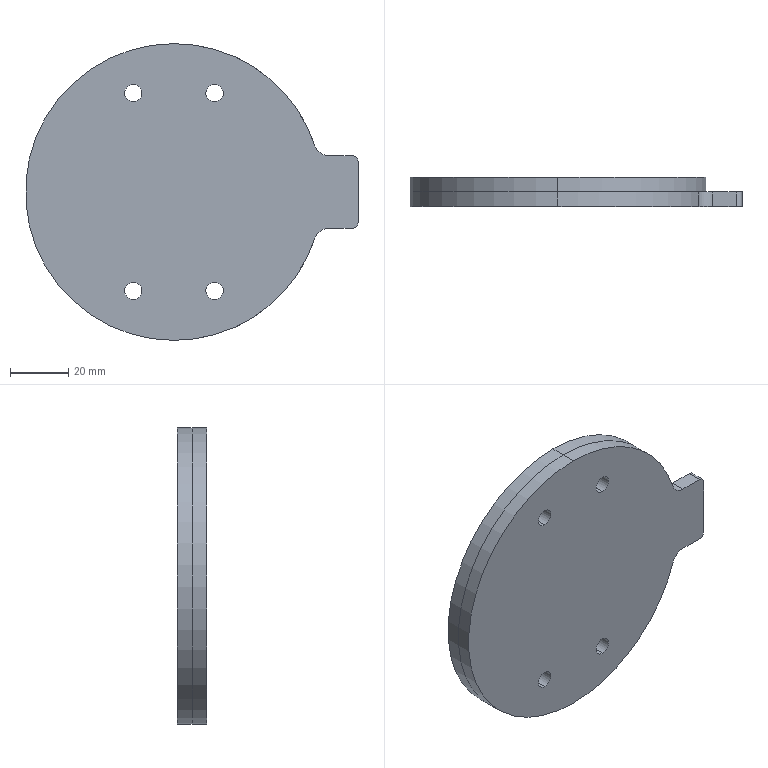Part | SolidWorks | features ICE 4, Extrusion 1, Fillet 1 | 2 solids | 41 faces | box 114.307 x 10 x 102 mm | volume 82051 mm3 | cylinder 31 | plane 10 | commonest cylinder face diameters 6 x16 8 x6 102 x5 4 x2 10 x2
STEP:
#1=CARTESIAN_POINT('',(-14.,0.,-37.));
#2=VERTEX_POINT('',#1);
#3=CARTESIAN_POINT('',(-14.,0.,-31.));
#4=VERTEX_POINT('',#3);
#5=CARTESIAN_POINT('',(-14.,0.,-34.));
#6=DIRECTION('',(0.,1.,0.));
#7=DIRECTION('',(0.,0.,1.));
#8=AXIS2_PLACEMENT_3D('',#5,#6,#7);
#9=CIRCLE('',#8,3.);
#10=EDGE_CURVE('',#2,#4,#9,.T.);
#11=ORIENTED_EDGE('',*,*,#10,.F.);
#12=CARTESIAN_POINT('',(-14.,5.,-37.));
#13=VERTEX_POINT('',#12);
#14=CARTESIAN_POINT('',(-14.,0.,-37.));
#15=DIRECTION('',(0.,1.,0.));
#16=VECTOR('',#15,1000.);
#17=LINE('',#14,#16);
#18=EDGE_CURVE('',#2,#13,#17,.T.);
#19=ORIENTED_EDGE('',*,*,#18,.T.);
#20=CARTESIAN_POINT('',(-14.,5.,-31.));
#21=VERTEX_POINT('',#20);
#22=CARTESIAN_POINT('',(-14.,5.,-34.));
#23=DIRECTION('',(0.,1.,0.));
#24=DIRECTION('',(0.,0.,1.));
#25=AXIS2_PLACEMENT_3D('',#22,#23,#24);
#26=CIRCLE('',#25,3.);
#27=EDGE_CURVE('',#13,#21,#26,.T.);
#28=ORIENTED_EDGE('',*,*,#27,.T.);
#29=CARTESIAN_POINT('',(-14.,0.,-31.));
#30=DIRECTION('',(0.,1.,0.));
#31=VECTOR('',#30,1000.);
#32=LINE('',#29,#31);
#33=EDGE_CURVE('',#4,#21,#32,.T.);
#34=ORIENTED_EDGE('',*,*,#33,.F.);
#35=EDGE_LOOP('',(#11,#19,#28,#34));
#36=FACE_OUTER_BOUND('',#35,.T.);
#37=CARTESIAN_POINT('',(-14.,0.,-34.));
#38=DIRECTION('',(0.,1.,0.));
#39=DIRECTION('',(0.,0.,1.));
#40=AXIS2_PLACEMENT_3D('',#37,#38,#39);
#41=CYLINDRICAL_SURFACE('',#40,3.);
#42=ADVANCED_FACE('',(#36),#41,.F.);
#43=CARTESIAN_POINT('',(14.,0.,-37.));
#44=VERTEX_POINT('',#43);
#45=CARTESIAN_POINT('',(14.,0.,-31.));
#46=VERTEX_POINT('',#45);
#47=CARTESIAN_POINT('',(14.,0.,-34.));
#48=DIRECTION('',(0.,1.,0.));
#49=DIRECTION('',(0.,0.,-1.));
#50=AXIS2_PLACEMENT_3D('',#47,#48,#49);
#51=CIRCLE('',#50,3.);
#52=EDGE_CURVE('',#44,#46,#51,.T.);
#53=ORIENTED_EDGE('',*,*,#52,.F.);
#54=CARTESIAN_POINT('',(14.,5.,-37.));
#55=VERTEX_POINT('',#54);
#56=CARTESIAN_POINT('',(14.,0.,-37.));
#57=DIRECTION('',(0.,1.,0.));
#58=VECTOR('',#57,1000.);
#59=LINE('',#56,#58);
#60=EDGE_CURVE('',#44,#55,#59,.T.);
#61=ORIENTED_EDGE('',*,*,#60,.T.);
#62=CARTESIAN_POINT('',(14.,5.,-31.));
#63=VERTEX_POINT('',#62);
#64=CARTESIAN_POINT('',(14.,5.,-34.));
#65=DIRECTION('',(0.,1.,0.));
#66=DIRECTION('',(0.,0.,1.));
#67=AXIS2_PLACEMENT_3D('',#64,#65,#66);
#68=CIRCLE('',#67,3.);
#69=EDGE_CURVE('',#55,#63,#68,.T.);
#70=ORIENTED_EDGE('',*,*,#69,.T.);
#71=CARTESIAN_POINT('',(14.,0.,-31.));
#72=DIRECTION('',(0.,1.,0.));
#73=VECTOR('',#72,1000.);
#74=LINE('',#71,#73);
#75=EDGE_CURVE('',#46,#63,#74,.T.);
#76=ORIENTED_EDGE('',*,*,#75,.F.);
#77=EDGE_LOOP('',(#53,#61,#70,#76));
#78=FACE_OUTER_BOUND('',#77,.T.);
#79=CARTESIAN_POINT('',(14.,0.,-34.));
#80=DIRECTION('',(0.,1.,0.));
#81=DIRECTION('',(0.,0.,1.));
#82=AXIS2_PLACEMENT_3D('',#79,#80,#81);
#83=CYLINDRICAL_SURFACE('',#82,3.);
#84=ADVANCED_FACE('',(#78),#83,.F.);
#85=CARTESIAN_POINT('',(14.,0.,31.));
#86=VERTEX_POINT('',#85);
#87=CARTESIAN_POINT('',(14.,0.,37.));
#88=VERTEX_POINT('',#87);
#89=CARTESIAN_POINT('',(14.,0.,34.));
#90=DIRECTION('',(0.,1.,0.));
#91=DIRECTION('',(0.,0.,1.));
#92=AXIS2_PLACEMENT_3D('',#89,#90,#91);
#93=CIRCLE('',#92,3.);
#94=EDGE_CURVE('',#86,#88,#93,.T.);
#95=ORIENTED_EDGE('',*,*,#94,.F.);
#96=CARTESIAN_POINT('',(14.,5.,31.));
#97=VERTEX_POINT('',#96);
#98=CARTESIAN_POINT('',(14.,0.,31.));
#99=DIRECTION('',(0.,1.,0.));
#100=VECTOR('',#99,1000.);
#101=LINE('',#98,#100);
#102=EDGE_CURVE('',#86,#97,#101,.T.);
#103=ORIENTED_EDGE('',*,*,#102,.T.);
#104=CARTESIAN_POINT('',(14.,5.,37.));
#105=VERTEX_POINT('',#104);
#106=CARTESIAN_POINT('',(14.,5.,34.));
#107=DIRECTION('',(0.,1.,0.));
#108=DIRECTION('',(0.,0.,1.));
#109=AXIS2_PLACEMENT_3D('',#106,#107,#108);
#110=CIRCLE('',#109,3.);
#111=EDGE_CURVE('',#97,#105,#110,.T.);
#112=ORIENTED_EDGE('',*,*,#111,.T.);
#113=CARTESIAN_POINT('',(14.,0.,37.));
#114=DIRECTION('',(0.,1.,0.));
#115=VECTOR('',#114,1000.);
#116=LINE('',#113,#115);
#117=EDGE_CURVE('',#88,#105,#116,.T.);
#118=ORIENTED_EDGE('',*,*,#117,.F.);
#119=EDGE_LOOP('',(#95,#103,#112,#118));
#120=FACE_OUTER_BOUND('',#119,.T.);
#121=CARTESIAN_POINT('',(14.,0.,34.));
#122=DIRECTION('',(0.,1.,0.));
#123=DIRECTION('',(0.,0.,1.));
#124=AXIS2_PLACEMENT_3D('',#121,#122,#123);
#125=CYLINDRICAL_SURFACE('',#124,3.);
#126=ADVANCED_FACE('',(#120),#125,.F.);
#127=CARTESIAN_POINT('',(-14.,0.,31.));
#128=VERTEX_POINT('',#127);
#129=CARTESIAN_POINT('',(-14.,0.,37.));
#130=VERTEX_POINT('',#129);
#131=CARTESIAN_POINT('',(-14.,0.,34.));
#132=DIRECTION('',(0.,1.,0.));
#133=DIRECTION('',(0.,0.,-1.));
#134=AXIS2_PLACEMENT_3D('',#131,#132,#133);
#135=CIRCLE('',#134,3.);
#136=EDGE_CURVE('',#128,#130,#135,.T.);
#137=ORIENTED_EDGE('',*,*,#136,.F.);
#138=CARTESIAN_POINT('',(-14.,5.,31.));
#139=VERTEX_POINT('',#138);
#140=CARTESIAN_POINT('',(-14.,0.,31.));
#141=DIRECTION('',(0.,1.,0.));
#142=VECTOR('',#141,1000.);
#143=LINE('',#140,#142);
#144=EDGE_CURVE('',#128,#139,#143,.T.);
#145=ORIENTED_EDGE('',*,*,#144,.T.);
#146=CARTESIAN_POINT('',(-14.,5.,37.));
#147=VERTEX_POINT('',#146);
#148=CARTESIAN_POINT('',(-14.,5.,34.));
#149=DIRECTION('',(0.,1.,0.));
#150=DIRECTION('',(0.,0.,1.));
#151=AXIS2_PLACEMENT_3D('',#148,#149,#150);
#152=CIRCLE('',#151,3.);
#153=EDGE_CURVE('',#139,#147,#152,.T.);
#154=ORIENTED_EDGE('',*,*,#153,.T.);
#155=CARTESIAN_POINT('',(-14.,0.,37.));
#156=DIRECTION('',(0.,1.,0.));
#157=VECTOR('',#156,1000.);
#158=LINE('',#155,#157);
#159=EDGE_CURVE('',#130,#147,#158,.T.);
#160=ORIENTED_EDGE('',*,*,#159,.F.);
#161=EDGE_LOOP('',(#137,#145,#154,#160));
#162=FACE_OUTER_BOUND('',#161,.T.);
#163=CARTESIAN_POINT('',(-14.,0.,34.));
#164=DIRECTION('',(0.,1.,0.));
#165=DIRECTION('',(0.,0.,1.));
#166=AXIS2_PLACEMENT_3D('',#163,#164,#165);
#167=CYLINDRICAL_SURFACE('',#166,3.);
#168=ADVANCED_FACE('',(#162),#167,.F.);
#169=CARTESIAN_POINT('',(0.,5.,51.));
#170=VERTEX_POINT('',#169);
#171=CARTESIAN_POINT('',(48.446,5.,15.938));
#172=VERTEX_POINT('',#171);
#173=CARTESIAN_POINT('',(0.,5.,0.));
#174=DIRECTION('',(0.,1.,0.));
#175=DIRECTION('',(0.,0.,1.));
#176=AXIS2_PLACEMENT_3D('',#173,#174,#175);
#177=CIRCLE('',#176,51.);
#178=EDGE_CURVE('',#170,#172,#177,.T.);
#179=ORIENTED_EDGE('',*,*,#178,.F.);
#180=CARTESIAN_POINT('',(0.,0.,51.));
#181=VERTEX_POINT('',#180);
#182=CARTESIAN_POINT('',(0.,5.,51.));
#183=DIRECTION('',(0.,-1.,0.));
#184=VECTOR('',#183,1000.);
#185=LINE('',#182,#184);
#186=EDGE_CURVE('',#170,#181,#185,.T.);
#187=ORIENTED_EDGE('',*,*,#186,.T.);
#188=CARTESIAN_POINT('',(48.446,0.,15.938));
#189=VERTEX_POINT('',#188);
#190=CARTESIAN_POINT('',(0.,0.,0.));
#191=DIRECTION('',(0.,1.,0.));
#192=DIRECTION('',(0.,0.,1.));
#193=AXIS2_PLACEMENT_3D('',#190,#191,#192);
#194=CIRCLE('',#193,51.);
#195=EDGE_CURVE('',#181,#189,#194,.T.);
#196=ORIENTED_EDGE('',*,*,#195,.T.);
#197=CARTESIAN_POINT('',(48.446,5.,15.938));
#198=DIRECTION('',(0.,1.,0.));
#199=VECTOR('',#198,1000.);
#200=LINE('',#197,#199);
#201=EDGE_CURVE('',#189,#172,#200,.T.);
#202=ORIENTED_EDGE('',*,*,#201,.T.);
#203=EDGE_LOOP('',(#179,#187,#196,#202));
#204=FACE_OUTER_BOUND('',#203,.T.);
#205=CARTESIAN_POINT('',(0.,5.,0.));
#206=DIRECTION('',(0.,-1.,0.));
#207=DIRECTION('',(0.,0.,-1.));
#208=AXIS2_PLACEMENT_3D('',#205,#206,#207);
#209=CYLINDRICAL_SURFACE('',#208,51.);
#210=ADVANCED_FACE('',(#204),#209,.T.);
#211=ORIENTED_EDGE('',*,*,#186,.F.);
#212=CARTESIAN_POINT('',(0.,5.,-51.));
#213=VERTEX_POINT('',#212);
#214=CARTESIAN_POINT('',(0.,5.,0.));
#215=DIRECTION('',(0.,1.,0.));
#216=DIRECTION('',(0.,0.,1.));
#217=AXIS2_PLACEMENT_3D('',#214,#215,#216);
#218=CIRCLE('',#217,51.);
#219=EDGE_CURVE('',#213,#170,#218,.T.);
#220=ORIENTED_EDGE('',*,*,#219,.F.);
#221=CARTESIAN_POINT('',(0.,0.,-51.));
#222=VERTEX_POINT('',#221);
#223=CARTESIAN_POINT('',(0.,5.,-51.));
#224=DIRECTION('',(0.,-1.,0.));
#225=VECTOR('',#224,1000.);
#226=LINE('',#223,#225);
#227=EDGE_CURVE('',#213,#222,#226,.T.);
#228=ORIENTED_EDGE('',*,*,#227,.T.);
#229=CARTESIAN_POINT('',(0.,0.,0.));
#230=DIRECTION('',(0.,1.,0.));
#231=DIRECTION('',(0.,0.,1.));
#232=AXIS2_PLACEMENT_3D('',#229,#230,#231);
#233=CIRCLE('',#232,51.);
#234=EDGE_CURVE('',#222,#181,#233,.T.);
#235=ORIENTED_EDGE('',*,*,#234,.T.);
#236=EDGE_LOOP('',(#211,#220,#228,#235));
#237=FACE_OUTER_BOUND('',#236,.T.);
#238=CARTESIAN_POINT('',(0.,5.,0.));
#239=DIRECTION('',(0.,-1.,0.));
#240=DIRECTION('',(0.,0.,-1.));
#241=AXIS2_PLACEMENT_3D('',#238,#239,#240);
#242=CYLINDRICAL_SURFACE('',#241,51.);
#243=ADVANCED_FACE('',(#237),#242,.T.);
#244=ORIENTED_EDGE('',*,*,#227,.F.);
#245=CARTESIAN_POINT('',(48.446,5.,-15.937));
#246=VERTEX_POINT('',#245);
#247=CARTESIAN_POINT('',(0.,5.,0.));
#248=DIRECTION('',(0.,1.,0.));
#249=DIRECTION('',(0.,0.,1.));
#250=AXIS2_PLACEMENT_3D('',#247,#248,#249);
#251=CIRCLE('',#250,51.);
#252=EDGE_CURVE('',#246,#213,#251,.T.);
#253=ORIENTED_EDGE('',*,*,#252,.F.);
#254=CARTESIAN_POINT('',(48.446,0.,-15.937));
#255=VERTEX_POINT('',#254);
#256=CARTESIAN_POINT('',(48.446,5.,-15.937));
#257=DIRECTION('',(0.,-1.,0.));
#258=VECTOR('',#257,1000.);
#259=LINE('',#256,#258);
#260=EDGE_CURVE('',#246,#255,#259,.T.);
#261=ORIENTED_EDGE('',*,*,#260,.T.);
#262=CARTESIAN_POINT('',(0.,0.,0.));
#263=DIRECTION('',(0.,1.,0.));
#264=DIRECTION('',(0.,0.,1.));
#265=AXIS2_PLACEMENT_3D('',#262,#263,#264);
#266=CIRCLE('',#265,51.);
#267=EDGE_CURVE('',#255,#222,#266,.T.);
#268=ORIENTED_EDGE('',*,*,#267,.T.);
#269=EDGE_LOOP('',(#244,#253,#261,#268));
#270=FACE_OUTER_BOUND('',#269,.T.);
#271=CARTESIAN_POINT('',(0.,5.,0.));
#272=DIRECTION('',(0.,-1.,0.));
#273=DIRECTION('',(0.,0.,-1.));
#274=AXIS2_PLACEMENT_3D('',#271,#272,#273);
#275=CYLINDRICAL_SURFACE('',#274,51.);
#276=ADVANCED_FACE('',(#270),#275,.T.);
#277=CARTESIAN_POINT('',(-14.,5.,-34.));
#278=DIRECTION('',(0.,1.,0.));
#279=DIRECTION('',(0.,0.,1.));
#280=AXIS2_PLACEMENT_3D('',#277,#278,#279);
#281=CIRCLE('',#280,3.);
#282=EDGE_CURVE('',#21,#13,#281,.T.);
#283=ORIENTED_EDGE('',*,*,#282,.F.);
#284=ORIENTED_EDGE('',*,*,#27,.F.);
#285=EDGE_LOOP('',(#283,#284));
#286=FACE_BOUND('',#285,.T.);
#287=CARTESIAN_POINT('',(14.,5.,-34.));
#288=DIRECTION('',(0.,1.,0.));
#289=DIRECTION('',(0.,0.,1.));
#290=AXIS2_PLACEMENT_3D('',#287,#288,#289);
#291=CIRCLE('',#290,3.);
#292=EDGE_CURVE('',#63,#55,#291,.T.);
#293=ORIENTED_EDGE('',*,*,#292,.F.);
#294=ORIENTED_EDGE('',*,*,#69,.F.);
#295=EDGE_LOOP('',(#293,#294));
#296=FACE_BOUND('',#295,.T.);
#297=CARTESIAN_POINT('',(14.,5.,34.));
#298=DIRECTION('',(0.,1.,0.));
#299=DIRECTION('',(0.,0.,1.));
#300=AXIS2_PLACEMENT_3D('',#297,#298,#299);
#301=CIRCLE('',#300,3.);
#302=EDGE_CURVE('',#105,#97,#301,.T.);
#303=ORIENTED_EDGE('',*,*,#302,.F.);
#304=ORIENTED_EDGE('',*,*,#111,.F.);
#305=EDGE_LOOP('',(#303,#304));
#306=FACE_BOUND('',#305,.T.);
#307=CARTESIAN_POINT('',(-14.,5.,34.));
#308=DIRECTION('',(0.,1.,0.));
#309=DIRECTION('',(0.,0.,1.));
#310=AXIS2_PLACEMENT_3D('',#307,#308,#309);
#311=CIRCLE('',#310,3.);
#312=EDGE_CURVE('',#147,#139,#311,.T.);
#313=ORIENTED_EDGE('',*,*,#312,.F.);
#314=ORIENTED_EDGE('',*,*,#153,.F.);
#315=EDGE_LOOP('',(#313,#314));
#316=FACE_BOUND('',#315,.T.);
#317=CARTESIAN_POINT('',(61.307,5.,-12.5));
#318=VERTEX_POINT('',#317);
#319=CARTESIAN_POINT('',(53.195,5.,-12.5));
#320=VERTEX_POINT('',#319);
#321=CARTESIAN_POINT('',(49.444,5.,-12.5));
#322=DIRECTION('',(-1.,0.,0.));
#323=VECTOR('',#322,1000.);
#324=LINE('',#321,#323);
#325=EDGE_CURVE('',#318,#320,#324,.T.);
#326=ORIENTED_EDGE('',*,*,#325,.T.);
#327=CARTESIAN_POINT('',(53.195,5.,-17.5));
#328=DIRECTION('',(0.,-1.,0.));
#329=DIRECTION('',(0.,0.,1.));
#330=AXIS2_PLACEMENT_3D('',#327,#328,#329);
#331=CIRCLE('',#330,5.);
#332=EDGE_CURVE('',#320,#246,#331,.T.);
#333=ORIENTED_EDGE('',*,*,#332,.T.);
#334=ORIENTED_EDGE('',*,*,#252,.T.);
#335=ORIENTED_EDGE('',*,*,#219,.T.);
#336=ORIENTED_EDGE('',*,*,#178,.T.);
#337=CARTESIAN_POINT('',(53.195,5.,12.5));
#338=VERTEX_POINT('',#337);
#339=CARTESIAN_POINT('',(53.195,5.,17.5));
#340=DIRECTION('',(0.,-1.,0.));
#341=DIRECTION('',(0.,0.,1.));
#342=AXIS2_PLACEMENT_3D('',#339,#340,#341);
#343=CIRCLE('',#342,5.);
#344=EDGE_CURVE('',#172,#338,#343,.T.);
#345=ORIENTED_EDGE('',*,*,#344,.T.);
#346=CARTESIAN_POINT('',(61.307,5.,12.5));
#347=VERTEX_POINT('',#346);
#348=CARTESIAN_POINT('',(61.307,5.,12.5));
#349=DIRECTION('',(1.,0.,0.));
#350=VECTOR('',#349,1000.);
#351=LINE('',#348,#350);
#352=EDGE_CURVE('',#338,#347,#351,.T.);
#353=ORIENTED_EDGE('',*,*,#352,.T.);
#354=CARTESIAN_POINT('',(63.307,5.,10.5));
#355=VERTEX_POINT('',#354);
#356=CARTESIAN_POINT('',(61.307,5.,10.5));
#357=DIRECTION('',(0.,1.,0.));
#358=DIRECTION('',(0.,0.,1.));
#359=AXIS2_PLACEMENT_3D('',#356,#357,#358);
#360=CIRCLE('',#359,2.);
#361=EDGE_CURVE('',#347,#355,#360,.T.);
#362=ORIENTED_EDGE('',*,*,#361,.T.);
#363=CARTESIAN_POINT('',(63.307,5.,-10.5));
#364=VERTEX_POINT('',#363);
#365=CARTESIAN_POINT('',(63.307,5.,-10.5));
#366=DIRECTION('',(0.,0.,-1.));
#367=VECTOR('',#366,1000.);
#368=LINE('',#365,#367);
#369=EDGE_CURVE('',#355,#364,#368,.T.);
#370=ORIENTED_EDGE('',*,*,#369,.T.);
#371=CARTESIAN_POINT('',(61.307,5.,-10.5));
#372=DIRECTION('',(0.,1.,0.));
#373=DIRECTION('',(0.,0.,1.));
#374=AXIS2_PLACEMENT_3D('',#371,#372,#373);
#375=CIRCLE('',#374,2.);
#376=EDGE_CURVE('',#364,#318,#375,.T.);
#377=ORIENTED_EDGE('',*,*,#376,.T.);
#378=EDGE_LOOP('',(#326,#333,#334,#335,#336,#345,#353,#362,#370,#377));
#379=FACE_OUTER_BOUND('',#378,.T.);
#380=CARTESIAN_POINT('',(0.,5.,0.));
#381=DIRECTION('',(0.,1.,0.));
#382=DIRECTION('',(0.,0.,1.));
#383=AXIS2_PLACEMENT_3D('',#380,#381,#382);
#384=PLANE('',#383);
#385=ADVANCED_FACE('',(#286,#296,#306,#316,#379),#384,.T.);
#386=CARTESIAN_POINT('',(-14.,0.,-34.));
#387=DIRECTION('',(0.,1.,0.));
#388=DIRECTION('',(0.,0.,1.));
#389=AXIS2_PLACEMENT_3D('',#386,#387,#388);
#390=CIRCLE('',#389,3.);
#391=EDGE_CURVE('',#4,#2,#390,.T.);
#392=ORIENTED_EDGE('',*,*,#391,.T.);
#393=ORIENTED_EDGE('',*,*,#10,.T.);
#394=EDGE_LOOP('',(#392,#393));
#395=FACE_BOUND('',#394,.T.);
#396=CARTESIAN_POINT('',(14.,0.,-34.));
#397=DIRECTION('',(0.,1.,0.));
#398=DIRECTION('',(0.,0.,-1.));
#399=AXIS2_PLACEMENT_3D('',#396,#397,#398);
#400=CIRCLE('',#399,3.);
#401=EDGE_CURVE('',#46,#44,#400,.T.);
#402=ORIENTED_EDGE('',*,*,#401,.T.);
#403=ORIENTED_EDGE('',*,*,#52,.T.);
#404=EDGE_LOOP('',(#402,#403));
#405=FACE_BOUND('',#404,.T.);
#406=CARTESIAN_POINT('',(14.,0.,34.));
#407=DIRECTION('',(0.,1.,0.));
#408=DIRECTION('',(0.,0.,1.));
#409=AXIS2_PLACEMENT_3D('',#406,#407,#408);
#410=CIRCLE('',#409,3.);
#411=EDGE_CURVE('',#88,#86,#410,.T.);
#412=ORIENTED_EDGE('',*,*,#411,.T.);
#413=ORIENTED_EDGE('',*,*,#94,.T.);
#414=EDGE_LOOP('',(#412,#413));
#415=FACE_BOUND('',#414,.T.);
#416=CARTESIAN_POINT('',(-14.,0.,34.));
#417=DIRECTION('',(0.,1.,0.));
#418=DIRECTION('',(0.,0.,-1.));
#419=AXIS2_PLACEMENT_3D('',#416,#417,#418);
#420=CIRCLE('',#419,3.);
#421=EDGE_CURVE('',#130,#128,#420,.T.);
#422=ORIENTED_EDGE('',*,*,#421,.T.);
#423=ORIENTED_EDGE('',*,*,#136,.T.);
#424=EDGE_LOOP('',(#422,#423));
#425=FACE_BOUND('',#424,.T.);
#426=ORIENTED_EDGE('',*,*,#267,.F.);
#427=CARTESIAN_POINT('',(53.195,0.,-12.5));
#428=VERTEX_POINT('',#427);
#429=CARTESIAN_POINT('',(53.195,0.,-17.5));
#430=DIRECTION('',(0.,1.,0.));
#431=DIRECTION('',(0.,0.,1.));
#432=AXIS2_PLACEMENT_3D('',#429,#430,#431);
#433=CIRCLE('',#432,5.);
#434=EDGE_CURVE('',#255,#428,#433,.T.);
#435=ORIENTED_EDGE('',*,*,#434,.T.);
#436=CARTESIAN_POINT('',(61.307,0.,-12.5));
#437=VERTEX_POINT('',#436);
#438=CARTESIAN_POINT('',(49.444,0.,-12.5));
#439=DIRECTION('',(-1.,0.,0.));
#440=VECTOR('',#439,1000.);
#441=LINE('',#438,#440);
#442=EDGE_CURVE('',#437,#428,#441,.T.);
#443=ORIENTED_EDGE('',*,*,#442,.F.);
#444=CARTESIAN_POINT('',(63.307,0.,-10.5));
#445=VERTEX_POINT('',#444);
#446=CARTESIAN_POINT('',(61.307,0.,-10.5));
#447=DIRECTION('',(0.,1.,0.));
#448=DIRECTION('',(0.,0.,1.));
#449=AXIS2_PLACEMENT_3D('',#446,#447,#448);
#450=CIRCLE('',#449,2.);
#451=EDGE_CURVE('',#445,#437,#450,.T.);
#452=ORIENTED_EDGE('',*,*,#451,.F.);
#453=CARTESIAN_POINT('',(63.307,0.,10.5));
#454=VERTEX_POINT('',#453);
#455=CARTESIAN_POINT('',(63.307,0.,-10.5));
#456=DIRECTION('',(0.,0.,-1.));
#457=VECTOR('',#456,1000.);
#458=LINE('',#455,#457);
#459=EDGE_CURVE('',#454,#445,#458,.T.);
#460=ORIENTED_EDGE('',*,*,#459,.F.);
#461=CARTESIAN_POINT('',(61.307,0.,12.5));
#462=VERTEX_POINT('',#461);
#463=CARTESIAN_POINT('',(61.307,0.,10.5));
#464=DIRECTION('',(0.,1.,0.));
#465=DIRECTION('',(0.,0.,1.));
#466=AXIS2_PLACEMENT_3D('',#463,#464,#465);
#467=CIRCLE('',#466,2.);
#468=EDGE_CURVE('',#462,#454,#467,.T.);
#469=ORIENTED_EDGE('',*,*,#468,.F.);
#470=CARTESIAN_POINT('',(53.195,0.,12.5));
#471=VERTEX_POINT('',#470);
#472=CARTESIAN_POINT('',(61.307,0.,12.5));
#473=DIRECTION('',(1.,0.,0.));
#474=VECTOR('',#473,1000.);
#475=LINE('',#472,#474);
#476=EDGE_CURVE('',#471,#462,#475,.T.);
#477=ORIENTED_EDGE('',*,*,#476,.F.);
#478=CARTESIAN_POINT('',(53.195,0.,17.5));
#479=DIRECTION('',(0.,1.,0.));
#480=DIRECTION('',(0.,0.,1.));
#481=AXIS2_PLACEMENT_3D('',#478,#479,#480);
#482=CIRCLE('',#481,5.);
#483=EDGE_CURVE('',#471,#189,#482,.T.);
#484=ORIENTED_EDGE('',*,*,#483,.T.);
#485=ORIENTED_EDGE('',*,*,#195,.F.);
#486=ORIENTED_EDGE('',*,*,#234,.F.);
#487=EDGE_LOOP('',(#426,#435,#443,#452,#460,#469,#477,#484,#485,#486));
#488=FACE_OUTER_BOUND('',#487,.T.);
#489=CARTESIAN_POINT('',(0.,0.,0.));
#490=DIRECTION('',(0.,1.,0.));
#491=DIRECTION('',(0.,0.,1.));
#492=AXIS2_PLACEMENT_3D('',#489,#490,#491);
#493=PLANE('',#492);
#494=ADVANCED_FACE('',(#395,#405,#415,#425,#488),#493,.F.);
#495=ORIENTED_EDGE('',*,*,#361,.F.);
#496=CARTESIAN_POINT('',(61.307,0.,12.5));
#497=DIRECTION('',(0.,1.,0.));
#498=VECTOR('',#497,1000.);
#499=LINE('',#496,#498);
#500=EDGE_CURVE('',#462,#347,#499,.T.);
#501=ORIENTED_EDGE('',*,*,#500,.F.);
#502=ORIENTED_EDGE('',*,*,#468,.T.);
#503=CARTESIAN_POINT('',(63.307,0.,10.5));
#504=DIRECTION('',(0.,1.,0.));
#505=VECTOR('',#504,1000.);
#506=LINE('',#503,#505);
#507=EDGE_CURVE('',#454,#355,#506,.T.);
#508=ORIENTED_EDGE('',*,*,#507,.T.);
#509=EDGE_LOOP('',(#495,#501,#502,#508));
#510=FACE_OUTER_BOUND('',#509,.T.);
#511=CARTESIAN_POINT('',(61.307,0.,10.5));
#512=DIRECTION('',(0.,1.,0.));
#513=DIRECTION('',(0.,0.,1.));
#514=AXIS2_PLACEMENT_3D('',#511,#512,#513);
#515=CYLINDRICAL_SURFACE('',#514,2.);
#516=ADVANCED_FACE('',(#510),#515,.T.);
#517=ORIENTED_EDGE('',*,*,#352,.F.);
#518=CARTESIAN_POINT('',(53.195,0.,12.5));
#519=DIRECTION('',(0.,-1.,0.));
#520=VECTOR('',#519,1000.);
#521=LINE('',#518,#520);
#522=EDGE_CURVE('',#338,#471,#521,.T.);
#523=ORIENTED_EDGE('',*,*,#522,.T.);
#524=ORIENTED_EDGE('',*,*,#476,.T.);
#525=ORIENTED_EDGE('',*,*,#500,.T.);
#526=EDGE_LOOP('',(#517,#523,#524,#525));
#527=FACE_OUTER_BOUND('',#526,.T.);
#528=CARTESIAN_POINT('',(61.307,0.,12.5));
#529=DIRECTION('',(0.,0.,1.));
#530=DIRECTION('',(1.,0.,0.));
#531=AXIS2_PLACEMENT_3D('',#528,#529,#530);
#532=PLANE('',#531);
#533=ADVANCED_FACE('',(#527),#532,.T.);
#534=ORIENTED_EDGE('',*,*,#442,.T.);
#535=CARTESIAN_POINT('',(53.195,0.,-12.5));
#536=DIRECTION('',(0.,1.,0.));
#537=VECTOR('',#536,1000.);
#538=LINE('',#535,#537);
#539=EDGE_CURVE('',#428,#320,#538,.T.);
#540=ORIENTED_EDGE('',*,*,#539,.T.);
#541=ORIENTED_EDGE('',*,*,#325,.F.);
#542=CARTESIAN_POINT('',(61.307,0.,-12.5));
#543=DIRECTION('',(0.,1.,0.));
#544=VECTOR('',#543,1000.);
#545=LINE('',#542,#544);
#546=EDGE_CURVE('',#437,#318,#545,.T.);
#547=ORIENTED_EDGE('',*,*,#546,.F.);
#548=EDGE_LOOP('',(#534,#540,#541,#547));
#549=FACE_OUTER_BOUND('',#548,.T.);
#550=CARTESIAN_POINT('',(49.444,0.,-12.5));
#551=DIRECTION('',(0.,0.,-1.));
#552=DIRECTION('',(-1.,0.,0.));
#553=AXIS2_PLACEMENT_3D('',#550,#551,#552);
#554=PLANE('',#553);
#555=ADVANCED_FACE('',(#549),#554,.T.);
#556=ORIENTED_EDGE('',*,*,#376,.F.);
#557=CARTESIAN_POINT('',(63.307,0.,-10.5));
#558=DIRECTION('',(0.,1.,0.));
#559=VECTOR('',#558,1000.);
#560=LINE('',#557,#559);
#561=EDGE_CURVE('',#445,#364,#560,.T.);
#562=ORIENTED_EDGE('',*,*,#561,.F.);
#563=ORIENTED_EDGE('',*,*,#451,.T.);
#564=ORIENTED_EDGE('',*,*,#546,.T.);
#565=EDGE_LOOP('',(#556,#562,#563,#564));
#566=FACE_OUTER_BOUND('',#565,.T.);
#567=CARTESIAN_POINT('',(61.307,0.,-10.5));
#568=DIRECTION('',(0.,1.,0.));
#569=DIRECTION('',(0.,0.,1.));
#570=AXIS2_PLACEMENT_3D('',#567,#568,#569);
#571=CYLINDRICAL_SURFACE('',#570,2.);
#572=ADVANCED_FACE('',(#566),#571,.T.);
#573=ORIENTED_EDGE('',*,*,#369,.F.);
#574=ORIENTED_EDGE('',*,*,#507,.F.);
#575=ORIENTED_EDGE('',*,*,#459,.T.);
#576=ORIENTED_EDGE('',*,*,#561,.T.);
#577=EDGE_LOOP('',(#573,#574,#575,#576));
#578=FACE_OUTER_BOUND('',#577,.T.);
#579=CARTESIAN_POINT('',(63.307,0.,-10.5));
#580=DIRECTION('',(1.,0.,0.));
#581=DIRECTION('',(0.,0.,-1.));
#582=AXIS2_PLACEMENT_3D('',#579,#580,#581);
#583=PLANE('',#582);
#584=ADVANCED_FACE('',(#578),#583,.T.);
#585=ORIENTED_EDGE('',*,*,#434,.F.);
#586=ORIENTED_EDGE('',*,*,#260,.F.);
#587=ORIENTED_EDGE('',*,*,#332,.F.);
#588=ORIENTED_EDGE('',*,*,#539,.F.);
#589=EDGE_LOOP('',(#585,#586,#587,#588));
#590=FACE_OUTER_BOUND('',#589,.T.);
#591=CARTESIAN_POINT('',(53.195,5.,-17.5));
#592=DIRECTION('',(0.,-1.,0.));
#593=DIRECTION('',(0.,0.,-1.));
#594=AXIS2_PLACEMENT_3D('',#591,#592,#593);
#595=CYLINDRICAL_SURFACE('',#594,5.);
#596=ADVANCED_FACE('',(#590),#595,.F.);
#597=ORIENTED_EDGE('',*,*,#483,.F.);
#598=ORIENTED_EDGE('',*,*,#522,.F.);
#599=ORIENTED_EDGE('',*,*,#344,.F.);
#600=ORIENTED_EDGE('',*,*,#201,.F.);
#601=EDGE_LOOP('',(#597,#598,#599,#600));
#602=FACE_OUTER_BOUND('',#601,.T.);
#603=CARTESIAN_POINT('',(53.195,5.,17.5));
#604=DIRECTION('',(0.,-1.,0.));
#605=DIRECTION('',(0.,0.,-1.));
#606=AXIS2_PLACEMENT_3D('',#603,#604,#605);
#607=CYLINDRICAL_SURFACE('',#606,5.);
#608=ADVANCED_FACE('',(#602),#607,.F.);
#609=ORIENTED_EDGE('',*,*,#144,.F.);
#610=ORIENTED_EDGE('',*,*,#421,.F.);
#611=ORIENTED_EDGE('',*,*,#159,.T.);
#612=ORIENTED_EDGE('',*,*,#312,.T.);
#613=EDGE_LOOP('',(#609,#610,#611,#612));
#614=FACE_OUTER_BOUND('',#613,.T.);
#615=CARTESIAN_POINT('',(-14.,0.,34.));
#616=DIRECTION('',(0.,1.,0.));
#617=DIRECTION('',(0.,0.,1.));
#618=AXIS2_PLACEMENT_3D('',#615,#616,#617);
#619=CYLINDRICAL_SURFACE('',#618,3.);
#620=ADVANCED_FACE('',(#614),#619,.F.);
#621=ORIENTED_EDGE('',*,*,#102,.F.);
#622=ORIENTED_EDGE('',*,*,#411,.F.);
#623=ORIENTED_EDGE('',*,*,#117,.T.);
#624=ORIENTED_EDGE('',*,*,#302,.T.);
#625=EDGE_LOOP('',(#621,#622,#623,#624));
#626=FACE_OUTER_BOUND('',#625,.T.);
#627=CARTESIAN_POINT('',(14.,0.,34.));
#628=DIRECTION('',(0.,1.,0.));
#629=DIRECTION('',(0.,0.,1.));
#630=AXIS2_PLACEMENT_3D('',#627,#628,#629);
#631=CYLINDRICAL_SURFACE('',#630,3.);
#632=ADVANCED_FACE('',(#626),#631,.F.);
#633=ORIENTED_EDGE('',*,*,#60,.F.);
#634=ORIENTED_EDGE('',*,*,#401,.F.);
#635=ORIENTED_EDGE('',*,*,#75,.T.);
#636=ORIENTED_EDGE('',*,*,#292,.T.);
#637=EDGE_LOOP('',(#633,#634,#635,#636));
#638=FACE_OUTER_BOUND('',#637,.T.);
#639=CARTESIAN_POINT('',(14.,0.,-34.));
#640=DIRECTION('',(0.,1.,0.));
#641=DIRECTION('',(0.,0.,1.));
#642=AXIS2_PLACEMENT_3D('',#639,#640,#641);
#643=CYLINDRICAL_SURFACE('',#642,3.);
#644=ADVANCED_FACE('',(#638),#643,.F.);
#645=ORIENTED_EDGE('',*,*,#18,.F.);
#646=ORIENTED_EDGE('',*,*,#391,.F.);
#647=ORIENTED_EDGE('',*,*,#33,.T.);
#648=ORIENTED_EDGE('',*,*,#282,.T.);
#649=EDGE_LOOP('',(#645,#646,#647,#648));
#650=FACE_OUTER_BOUND('',#649,.T.);
#651=CARTESIAN_POINT('',(-14.,0.,-34.));
#652=DIRECTION('',(0.,1.,0.));
#653=DIRECTION('',(0.,0.,1.));
#654=AXIS2_PLACEMENT_3D('',#651,#652,#653);
#655=CYLINDRICAL_SURFACE('',#654,3.);
#656=ADVANCED_FACE('',(#650),#655,.F.);
#657=CLOSED_SHELL('',(#42,#84,#126,#168,#210,#243,#276,#385,#494,#516,#533,#555,#572,#584,#596,#608,#620,#632,#644,#656));
#658=MANIFOLD_SOLID_BREP('',#657);
#659=CARTESIAN_POINT('',(-36.585,9.,-4.));
#660=VERTEX_POINT('',#659);
#661=CARTESIAN_POINT('',(-36.585,9.,4.));
#662=VERTEX_POINT('',#661);
#663=CARTESIAN_POINT('',(-36.585,9.,0.));
#664=DIRECTION('',(0.,1.,0.));
#665=DIRECTION('',(0.,0.,1.));
#666=AXIS2_PLACEMENT_3D('',#663,#664,#665);
#667=CIRCLE('',#666,4.);
#668=EDGE_CURVE('',#660,#662,#667,.T.);
#669=ORIENTED_EDGE('',*,*,#668,.F.);
#670=CARTESIAN_POINT('',(-36.585,10.,-4.));
#671=VERTEX_POINT('',#670);
#672=CARTESIAN_POINT('',(-36.585,9.,-4.));
#673=DIRECTION('',(0.,1.,0.));
#674=VECTOR('',#673,1000.);
#675=LINE('',#672,#674);
#676=EDGE_CURVE('',#660,#671,#675,.T.);
#677=ORIENTED_EDGE('',*,*,#676,.T.);
#678=CARTESIAN_POINT('',(-36.585,10.,4.));
#679=VERTEX_POINT('',#678);
#680=CARTESIAN_POINT('',(-36.585,10.,0.));
#681=DIRECTION('',(0.,1.,0.));
#682=DIRECTION('',(0.,0.,1.));
#683=AXIS2_PLACEMENT_3D('',#680,#681,#682);
#684=CIRCLE('',#683,4.);
#685=EDGE_CURVE('',#671,#679,#684,.T.);
#686=ORIENTED_EDGE('',*,*,#685,.T.);
#687=CARTESIAN_POINT('',(-36.585,9.,4.));
#688=DIRECTION('',(0.,1.,0.));
#689=VECTOR('',#688,1000.);
#690=LINE('',#687,#689);
#691=EDGE_CURVE('',#662,#679,#690,.T.);
#692=ORIENTED_EDGE('',*,*,#691,.F.);
#693=EDGE_LOOP('',(#669,#677,#686,#692));
#694=FACE_OUTER_BOUND('',#693,.T.);
#695=CARTESIAN_POINT('',(-36.585,9.,0.));
#696=DIRECTION('',(0.,1.,0.));
#697=DIRECTION('',(0.,0.,1.));
#698=AXIS2_PLACEMENT_3D('',#695,#696,#697);
#699=CYLINDRICAL_SURFACE('',#698,4.);
#700=ADVANCED_FACE('',(#694),#699,.F.);
#701=CARTESIAN_POINT('',(0.,9.,40.095));
#702=VERTEX_POINT('',#701);
#703=CARTESIAN_POINT('',(0.,9.,48.095));
#704=VERTEX_POINT('',#703);
#705=CARTESIAN_POINT('',(0.,9.,44.095));
#706=DIRECTION('',(0.,1.,0.));
#707=DIRECTION('',(0.,0.,1.));
#708=AXIS2_PLACEMENT_3D('',#705,#706,#707);
#709=CIRCLE('',#708,4.);
#710=EDGE_CURVE('',#702,#704,#709,.T.);
#711=ORIENTED_EDGE('',*,*,#710,.F.);
#712=CARTESIAN_POINT('',(0.,10.,40.095));
#713=VERTEX_POINT('',#712);
#714=CARTESIAN_POINT('',(0.,9.,40.095));
#715=DIRECTION('',(0.,1.,0.));
#716=VECTOR('',#715,1000.);
#717=LINE('',#714,#716);
#718=EDGE_CURVE('',#702,#713,#717,.T.);
#719=ORIENTED_EDGE('',*,*,#718,.T.);
#720=CARTESIAN_POINT('',(0.,10.,48.095));
#721=VERTEX_POINT('',#720);
#722=CARTESIAN_POINT('',(0.,10.,44.095));
#723=DIRECTION('',(0.,1.,0.));
#724=DIRECTION('',(0.,0.,1.));
#725=AXIS2_PLACEMENT_3D('',#722,#723,#724);
#726=CIRCLE('',#725,4.);
#727=EDGE_CURVE('',#713,#721,#726,.T.);
#728=ORIENTED_EDGE('',*,*,#727,.T.);
#729=CARTESIAN_POINT('',(0.,9.,48.095));
#730=DIRECTION('',(0.,1.,0.));
#731=VECTOR('',#730,1000.);
#732=LINE('',#729,#731);
#733=EDGE_CURVE('',#704,#721,#732,.T.);
#734=ORIENTED_EDGE('',*,*,#733,.F.);
#735=EDGE_LOOP('',(#711,#719,#728,#734));
#736=FACE_OUTER_BOUND('',#735,.T.);
#737=CARTESIAN_POINT('',(0.,9.,44.095));
#738=DIRECTION('',(0.,1.,0.));
#739=DIRECTION('',(0.,0.,1.));
#740=AXIS2_PLACEMENT_3D('',#737,#738,#739);
#741=CYLINDRICAL_SURFACE('',#740,4.);
#742=ADVANCED_FACE('',(#736),#741,.F.);
#743=CARTESIAN_POINT('',(0.,9.,-48.095));
#744=VERTEX_POINT('',#743);
#745=CARTESIAN_POINT('',(0.,9.,-40.095));
#746=VERTEX_POINT('',#745);
#747=CARTESIAN_POINT('',(0.,9.,-44.095));
#748=DIRECTION('',(0.,1.,0.));
#749=DIRECTION('',(0.,0.,-1.));
#750=AXIS2_PLACEMENT_3D('',#747,#748,#749);
#751=CIRCLE('',#750,4.);
#752=EDGE_CURVE('',#744,#746,#751,.T.);
#753=ORIENTED_EDGE('',*,*,#752,.F.);
#754=CARTESIAN_POINT('',(0.,10.,-48.095));
#755=VERTEX_POINT('',#754);
#756=CARTESIAN_POINT('',(0.,9.,-48.095));
#757=DIRECTION('',(0.,1.,0.));
#758=VECTOR('',#757,1000.);
#759=LINE('',#756,#758);
#760=EDGE_CURVE('',#744,#755,#759,.T.);
#761=ORIENTED_EDGE('',*,*,#760,.T.);
#762=CARTESIAN_POINT('',(0.,10.,-40.095));
#763=VERTEX_POINT('',#762);
#764=CARTESIAN_POINT('',(0.,10.,-44.095));
#765=DIRECTION('',(0.,1.,0.));
#766=DIRECTION('',(0.,0.,-1.));
#767=AXIS2_PLACEMENT_3D('',#764,#765,#766);
#768=CIRCLE('',#767,4.);
#769=EDGE_CURVE('',#755,#763,#768,.T.);
#770=ORIENTED_EDGE('',*,*,#769,.T.);
#771=CARTESIAN_POINT('',(0.,9.,-40.095));
#772=DIRECTION('',(0.,1.,0.));
#773=VECTOR('',#772,1000.);
#774=LINE('',#771,#773);
#775=EDGE_CURVE('',#746,#763,#774,.T.);
#776=ORIENTED_EDGE('',*,*,#775,.F.);
#777=EDGE_LOOP('',(#753,#761,#770,#776));
#778=FACE_OUTER_BOUND('',#777,.T.);
#779=CARTESIAN_POINT('',(0.,9.,-44.095));
#780=DIRECTION('',(0.,1.,0.));
#781=DIRECTION('',(0.,0.,1.));
#782=AXIS2_PLACEMENT_3D('',#779,#780,#781);
#783=CYLINDRICAL_SURFACE('',#782,4.);
#784=ADVANCED_FACE('',(#778),#783,.F.);
#785=CARTESIAN_POINT('',(-14.,5.,-37.));
#786=VERTEX_POINT('',#785);
#787=CARTESIAN_POINT('',(-14.,5.,-31.));
#788=VERTEX_POINT('',#787);
#789=CARTESIAN_POINT('',(-14.,5.,-34.));
#790=DIRECTION('',(0.,1.,0.));
#791=DIRECTION('',(0.,0.,1.));
#792=AXIS2_PLACEMENT_3D('',#789,#790,#791);
#793=CIRCLE('',#792,3.);
#794=EDGE_CURVE('',#786,#788,#793,.T.);
#795=ORIENTED_EDGE('',*,*,#794,.F.);
#796=CARTESIAN_POINT('',(-14.,10.,-37.));
#797=VERTEX_POINT('',#796);
#798=CARTESIAN_POINT('',(-14.,0.,-37.));
#799=DIRECTION('',(0.,1.,0.));
#800=VECTOR('',#799,1000.);
#801=LINE('',#798,#800);
#802=EDGE_CURVE('',#786,#797,#801,.T.);
#803=ORIENTED_EDGE('',*,*,#802,.T.);
#804=CARTESIAN_POINT('',(-14.,10.,-31.));
#805=VERTEX_POINT('',#804);
#806=CARTESIAN_POINT('',(-14.,10.,-34.));
#807=DIRECTION('',(0.,1.,0.));
#808=DIRECTION('',(0.,0.,1.));
#809=AXIS2_PLACEMENT_3D('',#806,#807,#808);
#810=CIRCLE('',#809,3.);
#811=EDGE_CURVE('',#797,#805,#810,.T.);
#812=ORIENTED_EDGE('',*,*,#811,.T.);
#813=CARTESIAN_POINT('',(-14.,0.,-31.));
#814=DIRECTION('',(0.,1.,0.));
#815=VECTOR('',#814,1000.);
#816=LINE('',#813,#815);
#817=EDGE_CURVE('',#788,#805,#816,.T.);
#818=ORIENTED_EDGE('',*,*,#817,.F.);
#819=EDGE_LOOP('',(#795,#803,#812,#818));
#820=FACE_OUTER_BOUND('',#819,.T.);
#821=CARTESIAN_POINT('',(-14.,0.,-34.));
#822=DIRECTION('',(0.,1.,0.));
#823=DIRECTION('',(0.,0.,1.));
#824=AXIS2_PLACEMENT_3D('',#821,#822,#823);
#825=CYLINDRICAL_SURFACE('',#824,3.);
#826=ADVANCED_FACE('',(#820),#825,.F.);
#827=CARTESIAN_POINT('',(14.,5.,-37.));
#828=VERTEX_POINT('',#827);
#829=CARTESIAN_POINT('',(14.,5.,-31.));
#830=VERTEX_POINT('',#829);
#831=CARTESIAN_POINT('',(14.,5.,-34.));
#832=DIRECTION('',(0.,1.,0.));
#833=DIRECTION('',(0.,0.,1.));
#834=AXIS2_PLACEMENT_3D('',#831,#832,#833);
#835=CIRCLE('',#834,3.);
#836=EDGE_CURVE('',#828,#830,#835,.T.);
#837=ORIENTED_EDGE('',*,*,#836,.F.);
#838=CARTESIAN_POINT('',(14.,10.,-37.));
#839=VERTEX_POINT('',#838);
#840=CARTESIAN_POINT('',(14.,0.,-37.));
#841=DIRECTION('',(0.,1.,0.));
#842=VECTOR('',#841,1000.);
#843=LINE('',#840,#842);
#844=EDGE_CURVE('',#828,#839,#843,.T.);
#845=ORIENTED_EDGE('',*,*,#844,.T.);
#846=CARTESIAN_POINT('',(14.,10.,-31.));
#847=VERTEX_POINT('',#846);
#848=CARTESIAN_POINT('',(14.,10.,-34.));
#849=DIRECTION('',(0.,1.,0.));
#850=DIRECTION('',(0.,0.,-1.));
#851=AXIS2_PLACEMENT_3D('',#848,#849,#850);
#852=CIRCLE('',#851,3.);
#853=EDGE_CURVE('',#839,#847,#852,.T.);
#854=ORIENTED_EDGE('',*,*,#853,.T.);
#855=CARTESIAN_POINT('',(14.,0.,-31.));
#856=DIRECTION('',(0.,1.,0.));
#857=VECTOR('',#856,1000.);
#858=LINE('',#855,#857);
#859=EDGE_CURVE('',#830,#847,#858,.T.);
#860=ORIENTED_EDGE('',*,*,#859,.F.);
#861=EDGE_LOOP('',(#837,#845,#854,#860));
#862=FACE_OUTER_BOUND('',#861,.T.);
#863=CARTESIAN_POINT('',(14.,0.,-34.));
#864=DIRECTION('',(0.,1.,0.));
#865=DIRECTION('',(0.,0.,1.));
#866=AXIS2_PLACEMENT_3D('',#863,#864,#865);
#867=CYLINDRICAL_SURFACE('',#866,3.);
#868=ADVANCED_FACE('',(#862),#867,.F.);
#869=CARTESIAN_POINT('',(14.,5.,31.));
#870=VERTEX_POINT('',#869);
#871=CARTESIAN_POINT('',(14.,5.,37.));
#872=VERTEX_POINT('',#871);
#873=CARTESIAN_POINT('',(14.,5.,34.));
#874=DIRECTION('',(0.,1.,0.));
#875=DIRECTION('',(0.,0.,1.));
#876=AXIS2_PLACEMENT_3D('',#873,#874,#875);
#877=CIRCLE('',#876,3.);
#878=EDGE_CURVE('',#870,#872,#877,.T.);
#879=ORIENTED_EDGE('',*,*,#878,.F.);
#880=CARTESIAN_POINT('',(14.,10.,31.));
#881=VERTEX_POINT('',#880);
#882=CARTESIAN_POINT('',(14.,0.,31.));
#883=DIRECTION('',(0.,1.,0.));
#884=VECTOR('',#883,1000.);
#885=LINE('',#882,#884);
#886=EDGE_CURVE('',#870,#881,#885,.T.);
#887=ORIENTED_EDGE('',*,*,#886,.T.);
#888=CARTESIAN_POINT('',(14.,10.,37.));
#889=VERTEX_POINT('',#888);
#890=CARTESIAN_POINT('',(14.,10.,34.));
#891=DIRECTION('',(0.,1.,0.));
#892=DIRECTION('',(0.,0.,1.));
#893=AXIS2_PLACEMENT_3D('',#890,#891,#892);
#894=CIRCLE('',#893,3.);
#895=EDGE_CURVE('',#881,#889,#894,.T.);
#896=ORIENTED_EDGE('',*,*,#895,.T.);
#897=CARTESIAN_POINT('',(14.,0.,37.));
#898=DIRECTION('',(0.,1.,0.));
#899=VECTOR('',#898,1000.);
#900=LINE('',#897,#899);
#901=EDGE_CURVE('',#872,#889,#900,.T.);
#902=ORIENTED_EDGE('',*,*,#901,.F.);
#903=EDGE_LOOP('',(#879,#887,#896,#902));
#904=FACE_OUTER_BOUND('',#903,.T.);
#905=CARTESIAN_POINT('',(14.,0.,34.));
#906=DIRECTION('',(0.,1.,0.));
#907=DIRECTION('',(0.,0.,1.));
#908=AXIS2_PLACEMENT_3D('',#905,#906,#907);
#909=CYLINDRICAL_SURFACE('',#908,3.);
#910=ADVANCED_FACE('',(#904),#909,.F.);
#911=CARTESIAN_POINT('',(-14.,5.,31.));
#912=VERTEX_POINT('',#911);
#913=CARTESIAN_POINT('',(-14.,5.,37.));
#914=VERTEX_POINT('',#913);
#915=CARTESIAN_POINT('',(-14.,5.,34.));
#916=DIRECTION('',(0.,1.,0.));
#917=DIRECTION('',(0.,0.,1.));
#918=AXIS2_PLACEMENT_3D('',#915,#916,#917);
#919=CIRCLE('',#918,3.);
#920=EDGE_CURVE('',#912,#914,#919,.T.);
#921=ORIENTED_EDGE('',*,*,#920,.F.);
#922=CARTESIAN_POINT('',(-14.,10.,31.));
#923=VERTEX_POINT('',#922);
#924=CARTESIAN_POINT('',(-14.,0.,31.));
#925=DIRECTION('',(0.,1.,0.));
#926=VECTOR('',#925,1000.);
#927=LINE('',#924,#926);
#928=EDGE_CURVE('',#912,#923,#927,.T.);
#929=ORIENTED_EDGE('',*,*,#928,.T.);
#930=CARTESIAN_POINT('',(-14.,10.,37.));
#931=VERTEX_POINT('',#930);
#932=CARTESIAN_POINT('',(-14.,10.,34.));
#933=DIRECTION('',(0.,1.,0.));
#934=DIRECTION('',(0.,0.,-1.));
#935=AXIS2_PLACEMENT_3D('',#932,#933,#934);
#936=CIRCLE('',#935,3.);
#937=EDGE_CURVE('',#923,#931,#936,.T.);
#938=ORIENTED_EDGE('',*,*,#937,.T.);
#939=CARTESIAN_POINT('',(-14.,0.,37.));
#940=DIRECTION('',(0.,1.,0.));
#941=VECTOR('',#940,1000.);
#942=LINE('',#939,#941);
#943=EDGE_CURVE('',#914,#931,#942,.T.);
#944=ORIENTED_EDGE('',*,*,#943,.F.);
#945=EDGE_LOOP('',(#921,#929,#938,#944));
#946=FACE_OUTER_BOUND('',#945,.T.);
#947=CARTESIAN_POINT('',(-14.,0.,34.));
#948=DIRECTION('',(0.,1.,0.));
#949=DIRECTION('',(0.,0.,1.));
#950=AXIS2_PLACEMENT_3D('',#947,#948,#949);
#951=CYLINDRICAL_SURFACE('',#950,3.);
#952=ADVANCED_FACE('',(#946),#951,.F.);
#953=CARTESIAN_POINT('',(0.,10.,51.));
#954=VERTEX_POINT('',#953);
#955=CARTESIAN_POINT('',(0.,10.,-51.));
#956=VERTEX_POINT('',#955);
#957=CARTESIAN_POINT('',(0.,10.,0.));
#958=DIRECTION('',(0.,1.,0.));
#959=DIRECTION('',(0.,0.,1.));
#960=AXIS2_PLACEMENT_3D('',#957,#958,#959);
#961=CIRCLE('',#960,51.);
#962=EDGE_CURVE('',#954,#956,#961,.T.);
#963=ORIENTED_EDGE('',*,*,#962,.F.);
#964=CARTESIAN_POINT('',(0.,5.,51.));
#965=VERTEX_POINT('',#964);
#966=CARTESIAN_POINT('',(0.,10.,51.));
#967=DIRECTION('',(0.,-1.,0.));
#968=VECTOR('',#967,1000.);
#969=LINE('',#966,#968);
#970=EDGE_CURVE('',#954,#965,#969,.T.);
#971=ORIENTED_EDGE('',*,*,#970,.T.);
#972=CARTESIAN_POINT('',(0.,5.,-51.));
#973=VERTEX_POINT('',#972);
#974=CARTESIAN_POINT('',(0.,5.,0.));
#975=DIRECTION('',(0.,1.,0.));
#976=DIRECTION('',(0.,0.,1.));
#977=AXIS2_PLACEMENT_3D('',#974,#975,#976);
#978=CIRCLE('',#977,51.);
#979=EDGE_CURVE('',#965,#973,#978,.T.);
#980=ORIENTED_EDGE('',*,*,#979,.T.);
#981=CARTESIAN_POINT('',(0.,10.,-51.));
#982=DIRECTION('',(0.,-1.,0.));
#983=VECTOR('',#982,1000.);
#984=LINE('',#981,#983);
#985=EDGE_CURVE('',#956,#973,#984,.T.);
#986=ORIENTED_EDGE('',*,*,#985,.F.);
#987=EDGE_LOOP('',(#963,#971,#980,#986));
#988=FACE_OUTER_BOUND('',#987,.T.);
#989=CARTESIAN_POINT('',(0.,10.,0.));
#990=DIRECTION('',(0.,-1.,0.));
#991=DIRECTION('',(0.,0.,-1.));
#992=AXIS2_PLACEMENT_3D('',#989,#990,#991);
#993=CYLINDRICAL_SURFACE('',#992,51.);
#994=ADVANCED_FACE('',(#988),#993,.T.);
#995=ORIENTED_EDGE('',*,*,#970,.F.);
#996=CARTESIAN_POINT('',(0.,10.,0.));
#997=DIRECTION('',(0.,1.,0.));
#998=DIRECTION('',(0.,0.,1.));
#999=AXIS2_PLACEMENT_3D('',#996,#997,#998);
#1000=CIRCLE('',#999,51.);
#1001=EDGE_CURVE('',#956,#954,#1000,.T.);
#1002=ORIENTED_EDGE('',*,*,#1001,.F.);
#1003=ORIENTED_EDGE('',*,*,#985,.T.);
#1004=CARTESIAN_POINT('',(0.,5.,0.));
#1005=DIRECTION('',(0.,1.,0.));
#1006=DIRECTION('',(0.,0.,1.));
#1007=AXIS2_PLACEMENT_3D('',#1004,#1005,#1006);
#1008=CIRCLE('',#1007,51.);
#1009=EDGE_CURVE('',#973,#965,#1008,.T.);
#1010=ORIENTED_EDGE('',*,*,#1009,.T.);
#1011=EDGE_LOOP('',(#995,#1002,#1003,#1010));
#1012=FACE_OUTER_BOUND('',#1011,.T.);
#1013=CARTESIAN_POINT('',(0.,10.,0.));
#1014=DIRECTION('',(0.,-1.,0.));
#1015=DIRECTION('',(0.,0.,-1.));
#1016=AXIS2_PLACEMENT_3D('',#1013,#1014,#1015);
#1017=CYLINDRICAL_SURFACE('',#1016,51.);
#1018=ADVANCED_FACE('',(#1012),#1017,.T.);
#1019=CARTESIAN_POINT('',(-36.585,10.,0.));
#1020=DIRECTION('',(0.,1.,0.));
#1021=DIRECTION('',(0.,0.,1.));
#1022=AXIS2_PLACEMENT_3D('',#1019,#1020,#1021);
#1023=CIRCLE('',#1022,4.);
#1024=EDGE_CURVE('',#679,#671,#1023,.T.);
#1025=ORIENTED_EDGE('',*,*,#1024,.F.);
#1026=ORIENTED_EDGE('',*,*,#685,.F.);
#1027=EDGE_LOOP('',(#1025,#1026));
#1028=FACE_BOUND('',#1027,.T.);
#1029=CARTESIAN_POINT('',(0.,10.,44.095));
#1030=DIRECTION('',(0.,1.,0.));
#1031=DIRECTION('',(0.,0.,1.));
#1032=AXIS2_PLACEMENT_3D('',#1029,#1030,#1031);
#1033=CIRCLE('',#1032,4.);
#1034=EDGE_CURVE('',#721,#713,#1033,.T.);
#1035=ORIENTED_EDGE('',*,*,#1034,.F.);
#1036=ORIENTED_EDGE('',*,*,#727,.F.);
#1037=EDGE_LOOP('',(#1035,#1036));
#1038=FACE_BOUND('',#1037,.T.);
#1039=CARTESIAN_POINT('',(0.,10.,-44.095));
#1040=DIRECTION('',(0.,1.,0.));
#1041=DIRECTION('',(0.,0.,-1.));
#1042=AXIS2_PLACEMENT_3D('',#1039,#1040,#1041);
#1043=CIRCLE('',#1042,4.);
#1044=EDGE_CURVE('',#763,#755,#1043,.T.);
#1045=ORIENTED_EDGE('',*,*,#1044,.F.);
#1046=ORIENTED_EDGE('',*,*,#769,.F.);
#1047=EDGE_LOOP('',(#1045,#1046));
#1048=FACE_BOUND('',#1047,.T.);
#1049=CARTESIAN_POINT('',(-14.,10.,-34.));
#1050=DIRECTION('',(0.,1.,0.));
#1051=DIRECTION('',(0.,0.,1.));
#1052=AXIS2_PLACEMENT_3D('',#1049,#1050,#1051);
#1053=CIRCLE('',#1052,3.);
#1054=EDGE_CURVE('',#805,#797,#1053,.T.);
#1055=ORIENTED_EDGE('',*,*,#1054,.F.);
#1056=ORIENTED_EDGE('',*,*,#811,.F.);
#1057=EDGE_LOOP('',(#1055,#1056));
#1058=FACE_BOUND('',#1057,.T.);
#1059=CARTESIAN_POINT('',(14.,10.,-34.));
#1060=DIRECTION('',(0.,1.,0.));
#1061=DIRECTION('',(0.,0.,-1.));
#1062=AXIS2_PLACEMENT_3D('',#1059,#1060,#1061);
#1063=CIRCLE('',#1062,3.);
#1064=EDGE_CURVE('',#847,#839,#1063,.T.);
#1065=ORIENTED_EDGE('',*,*,#1064,.F.);
#1066=ORIENTED_EDGE('',*,*,#853,.F.);
#1067=EDGE_LOOP('',(#1065,#1066));
#1068=FACE_BOUND('',#1067,.T.);
#1069=CARTESIAN_POINT('',(14.,10.,34.));
#1070=DIRECTION('',(0.,1.,0.));
#1071=DIRECTION('',(0.,0.,1.));
#1072=AXIS2_PLACEMENT_3D('',#1069,#1070,#1071);
#1073=CIRCLE('',#1072,3.);
#1074=EDGE_CURVE('',#889,#881,#1073,.T.);
#1075=ORIENTED_EDGE('',*,*,#1074,.F.);
#1076=ORIENTED_EDGE('',*,*,#895,.F.);
#1077=EDGE_LOOP('',(#1075,#1076));
#1078=FACE_BOUND('',#1077,.T.);
#1079=CARTESIAN_POINT('',(-14.,10.,34.));
#1080=DIRECTION('',(0.,1.,0.));
#1081=DIRECTION('',(0.,0.,-1.));
#1082=AXIS2_PLACEMENT_3D('',#1079,#1080,#1081);
#1083=CIRCLE('',#1082,3.);
#1084=EDGE_CURVE('',#931,#923,#1083,.T.);
#1085=ORIENTED_EDGE('',*,*,#1084,.F.);
#1086=ORIENTED_EDGE('',*,*,#937,.F.);
#1087=EDGE_LOOP('',(#1085,#1086));
#1088=FACE_BOUND('',#1087,.T.);
#1089=ORIENTED_EDGE('',*,*,#1001,.T.);
#1090=ORIENTED_EDGE('',*,*,#962,.T.);
#1091=EDGE_LOOP('',(#1089,#1090));
#1092=FACE_OUTER_BOUND('',#1091,.T.);
#1093=CARTESIAN_POINT('',(0.,10.,0.));
#1094=DIRECTION('',(0.,1.,0.));
#1095=DIRECTION('',(0.,0.,1.));
#1096=AXIS2_PLACEMENT_3D('',#1093,#1094,#1095);
#1097=PLANE('',#1096);
#1098=ADVANCED_FACE('',(#1028,#1038,#1048,#1058,#1068,#1078,#1088,#1092),#1097,.T.);
#1099=CARTESIAN_POINT('',(-14.,5.,-34.));
#1100=DIRECTION('',(0.,1.,0.));
#1101=DIRECTION('',(0.,0.,1.));
#1102=AXIS2_PLACEMENT_3D('',#1099,#1100,#1101);
#1103=CIRCLE('',#1102,3.);
#1104=EDGE_CURVE('',#788,#786,#1103,.T.);
#1105=ORIENTED_EDGE('',*,*,#1104,.T.);
#1106=ORIENTED_EDGE('',*,*,#794,.T.);
#1107=EDGE_LOOP('',(#1105,#1106));
#1108=FACE_BOUND('',#1107,.T.);
#1109=CARTESIAN_POINT('',(14.,5.,-34.));
#1110=DIRECTION('',(0.,1.,0.));
#1111=DIRECTION('',(0.,0.,1.));
#1112=AXIS2_PLACEMENT_3D('',#1109,#1110,#1111);
#1113=CIRCLE('',#1112,3.);
#1114=EDGE_CURVE('',#830,#828,#1113,.T.);
#1115=ORIENTED_EDGE('',*,*,#1114,.T.);
#1116=ORIENTED_EDGE('',*,*,#836,.T.);
#1117=EDGE_LOOP('',(#1115,#1116));
#1118=FACE_BOUND('',#1117,.T.);
#1119=CARTESIAN_POINT('',(14.,5.,34.));
#1120=DIRECTION('',(0.,1.,0.));
#1121=DIRECTION('',(0.,0.,1.));
#1122=AXIS2_PLACEMENT_3D('',#1119,#1120,#1121);
#1123=CIRCLE('',#1122,3.);
#1124=EDGE_CURVE('',#872,#870,#1123,.T.);
#1125=ORIENTED_EDGE('',*,*,#1124,.T.);
#1126=ORIENTED_EDGE('',*,*,#878,.T.);
#1127=EDGE_LOOP('',(#1125,#1126));
#1128=FACE_BOUND('',#1127,.T.);
#1129=CARTESIAN_POINT('',(-14.,5.,34.));
#1130=DIRECTION('',(0.,1.,0.));
#1131=DIRECTION('',(0.,0.,1.));
#1132=AXIS2_PLACEMENT_3D('',#1129,#1130,#1131);
#1133=CIRCLE('',#1132,3.);
#1134=EDGE_CURVE('',#914,#912,#1133,.T.);
#1135=ORIENTED_EDGE('',*,*,#1134,.T.);
#1136=ORIENTED_EDGE('',*,*,#920,.T.);
#1137=EDGE_LOOP('',(#1135,#1136));
#1138=FACE_BOUND('',#1137,.T.);
#1139=ORIENTED_EDGE('',*,*,#1009,.F.);
#1140=ORIENTED_EDGE('',*,*,#979,.F.);
#1141=EDGE_LOOP('',(#1139,#1140));
#1142=FACE_OUTER_BOUND('',#1141,.T.);
#1143=CARTESIAN_POINT('',(0.,5.,0.));
#1144=DIRECTION('',(0.,1.,0.));
#1145=DIRECTION('',(0.,0.,1.));
#1146=AXIS2_PLACEMENT_3D('',#1143,#1144,#1145);
#1147=PLANE('',#1146);
#1148=ADVANCED_FACE('',(#1108,#1118,#1128,#1138,#1142),#1147,.F.);
#1149=ORIENTED_EDGE('',*,*,#928,.F.);
#1150=ORIENTED_EDGE('',*,*,#1134,.F.);
#1151=ORIENTED_EDGE('',*,*,#943,.T.);
#1152=ORIENTED_EDGE('',*,*,#1084,.T.);
#1153=EDGE_LOOP('',(#1149,#1150,#1151,#1152));
#1154=FACE_OUTER_BOUND('',#1153,.T.);
#1155=CARTESIAN_POINT('',(-14.,0.,34.));
#1156=DIRECTION('',(0.,1.,0.));
#1157=DIRECTION('',(0.,0.,1.));
#1158=AXIS2_PLACEMENT_3D('',#1155,#1156,#1157);
#1159=CYLINDRICAL_SURFACE('',#1158,3.);
#1160=ADVANCED_FACE('',(#1154),#1159,.F.);
#1161=ORIENTED_EDGE('',*,*,#886,.F.);
#1162=ORIENTED_EDGE('',*,*,#1124,.F.);
#1163=ORIENTED_EDGE('',*,*,#901,.T.);
#1164=ORIENTED_EDGE('',*,*,#1074,.T.);
#1165=EDGE_LOOP('',(#1161,#1162,#1163,#1164));
#1166=FACE_OUTER_BOUND('',#1165,.T.);
#1167=CARTESIAN_POINT('',(14.,0.,34.));
#1168=DIRECTION('',(0.,1.,0.));
#1169=DIRECTION('',(0.,0.,1.));
#1170=AXIS2_PLACEMENT_3D('',#1167,#1168,#1169);
#1171=CYLINDRICAL_SURFACE('',#1170,3.);
#1172=ADVANCED_FACE('',(#1166),#1171,.F.);
#1173=ORIENTED_EDGE('',*,*,#844,.F.);
#1174=ORIENTED_EDGE('',*,*,#1114,.F.);
#1175=ORIENTED_EDGE('',*,*,#859,.T.);
#1176=ORIENTED_EDGE('',*,*,#1064,.T.);
#1177=EDGE_LOOP('',(#1173,#1174,#1175,#1176));
#1178=FACE_OUTER_BOUND('',#1177,.T.);
#1179=CARTESIAN_POINT('',(14.,0.,-34.));
#1180=DIRECTION('',(0.,1.,0.));
#1181=DIRECTION('',(0.,0.,1.));
#1182=AXIS2_PLACEMENT_3D('',#1179,#1180,#1181);
#1183=CYLINDRICAL_SURFACE('',#1182,3.);
#1184=ADVANCED_FACE('',(#1178),#1183,.F.);
#1185=ORIENTED_EDGE('',*,*,#802,.F.);
#1186=ORIENTED_EDGE('',*,*,#1104,.F.);
#1187=ORIENTED_EDGE('',*,*,#817,.T.);
#1188=ORIENTED_EDGE('',*,*,#1054,.T.);
#1189=EDGE_LOOP('',(#1185,#1186,#1187,#1188));
#1190=FACE_OUTER_BOUND('',#1189,.T.);
#1191=CARTESIAN_POINT('',(-14.,0.,-34.));
#1192=DIRECTION('',(0.,1.,0.));
#1193=DIRECTION('',(0.,0.,1.));
#1194=AXIS2_PLACEMENT_3D('',#1191,#1192,#1193);
#1195=CYLINDRICAL_SURFACE('',#1194,3.);
#1196=ADVANCED_FACE('',(#1190),#1195,.F.);
#1197=ORIENTED_EDGE('',*,*,#760,.F.);
#1198=CARTESIAN_POINT('',(0.,9.,-44.095));
#1199=DIRECTION('',(0.,1.,0.));
#1200=DIRECTION('',(0.,0.,-1.));
#1201=AXIS2_PLACEMENT_3D('',#1198,#1199,#1200);
#1202=CIRCLE('',#1201,4.);
#1203=EDGE_CURVE('',#746,#744,#1202,.T.);
#1204=ORIENTED_EDGE('',*,*,#1203,.F.);
#1205=ORIENTED_EDGE('',*,*,#775,.T.);
#1206=ORIENTED_EDGE('',*,*,#1044,.T.);
#1207=EDGE_LOOP('',(#1197,#1204,#1205,#1206));
#1208=FACE_OUTER_BOUND('',#1207,.T.);
#1209=CARTESIAN_POINT('',(0.,9.,-44.095));
#1210=DIRECTION('',(0.,1.,0.));
#1211=DIRECTION('',(0.,0.,1.));
#1212=AXIS2_PLACEMENT_3D('',#1209,#1210,#1211);
#1213=CYLINDRICAL_SURFACE('',#1212,4.);
#1214=ADVANCED_FACE('',(#1208),#1213,.F.);
#1215=ORIENTED_EDGE('',*,*,#1203,.T.);
#1216=ORIENTED_EDGE('',*,*,#752,.T.);
#1217=EDGE_LOOP('',(#1215,#1216));
#1218=FACE_OUTER_BOUND('',#1217,.T.);
#1219=CARTESIAN_POINT('',(0.,9.,-44.095));
#1220=DIRECTION('',(0.,-1.,0.));
#1221=DIRECTION('',(0.,0.,-1.));
#1222=AXIS2_PLACEMENT_3D('',#1219,#1220,#1221);
#1223=PLANE('',#1222);
#1224=ADVANCED_FACE('',(#1218),#1223,.F.);
#1225=ORIENTED_EDGE('',*,*,#718,.F.);
#1226=CARTESIAN_POINT('',(0.,9.,44.095));
#1227=DIRECTION('',(0.,1.,0.));
#1228=DIRECTION('',(0.,0.,1.));
#1229=AXIS2_PLACEMENT_3D('',#1226,#1227,#1228);
#1230=CIRCLE('',#1229,4.);
#1231=EDGE_CURVE('',#704,#702,#1230,.T.);
#1232=ORIENTED_EDGE('',*,*,#1231,.F.);
#1233=ORIENTED_EDGE('',*,*,#733,.T.);
#1234=ORIENTED_EDGE('',*,*,#1034,.T.);
#1235=EDGE_LOOP('',(#1225,#1232,#1233,#1234));
#1236=FACE_OUTER_BOUND('',#1235,.T.);
#1237=CARTESIAN_POINT('',(0.,9.,44.095));
#1238=DIRECTION('',(0.,1.,0.));
#1239=DIRECTION('',(0.,0.,1.));
#1240=AXIS2_PLACEMENT_3D('',#1237,#1238,#1239);
#1241=CYLINDRICAL_SURFACE('',#1240,4.);
#1242=ADVANCED_FACE('',(#1236),#1241,.F.);
#1243=ORIENTED_EDGE('',*,*,#1231,.T.);
#1244=ORIENTED_EDGE('',*,*,#710,.T.);
#1245=EDGE_LOOP('',(#1243,#1244));
#1246=FACE_OUTER_BOUND('',#1245,.T.);
#1247=CARTESIAN_POINT('',(0.,9.,44.095));
#1248=DIRECTION('',(0.,1.,0.));
#1249=DIRECTION('',(0.,0.,1.));
#1250=AXIS2_PLACEMENT_3D('',#1247,#1248,#1249);
#1251=PLANE('',#1250);
#1252=ADVANCED_FACE('',(#1246),#1251,.T.);
#1253=ORIENTED_EDGE('',*,*,#676,.F.);
#1254=CARTESIAN_POINT('',(-36.585,9.,0.));
#1255=DIRECTION('',(0.,1.,0.));
#1256=DIRECTION('',(0.,0.,1.));
#1257=AXIS2_PLACEMENT_3D('',#1254,#1255,#1256);
#1258=CIRCLE('',#1257,4.);
#1259=EDGE_CURVE('',#662,#660,#1258,.T.);
#1260=ORIENTED_EDGE('',*,*,#1259,.F.);
#1261=ORIENTED_EDGE('',*,*,#691,.T.);
#1262=ORIENTED_EDGE('',*,*,#1024,.T.);
#1263=EDGE_LOOP('',(#1253,#1260,#1261,#1262));
#1264=FACE_OUTER_BOUND('',#1263,.T.);
#1265=CARTESIAN_POINT('',(-36.585,9.,0.));
#1266=DIRECTION('',(0.,1.,0.));
#1267=DIRECTION('',(0.,0.,1.));
#1268=AXIS2_PLACEMENT_3D('',#1265,#1266,#1267);
#1269=CYLINDRICAL_SURFACE('',#1268,4.);
#1270=ADVANCED_FACE('',(#1264),#1269,.F.);
#1271=ORIENTED_EDGE('',*,*,#1259,.T.);
#1272=ORIENTED_EDGE('',*,*,#668,.T.);
#1273=EDGE_LOOP('',(#1271,#1272));
#1274=FACE_OUTER_BOUND('',#1273,.T.);
#1275=CARTESIAN_POINT('',(-36.585,9.,0.));
#1276=DIRECTION('',(0.,1.,0.));
#1277=DIRECTION('',(0.,0.,1.));
#1278=AXIS2_PLACEMENT_3D('',#1275,#1276,#1277);
#1279=PLANE('',#1278);
#1280=ADVANCED_FACE('',(#1274),#1279,.T.);
#1281=CLOSED_SHELL('',(#700,#742,#784,#826,#868,#910,#952,#994,#1018,#1098,#1148,#1160,#1172,#1184,#1196,#1214,#1224,#1242,#1252,#1270,#1280));
#1282=MANIFOLD_SOLID_BREP('',#1281);
#1283=CARTESIAN_POINT('',(0.,0.,0.));
#1284=DIRECTION('',(0.,0.,1.));
#1285=DIRECTION('',(1.,0.,0.));
#1286=AXIS2_PLACEMENT_3D('',#1283,#1284,#1285);
#1287=(LENGTH_UNIT()NAMED_UNIT(*)SI_UNIT(.MILLI.,.METRE.));
#1288=UNCERTAINTY_MEASURE_WITH_UNIT(LENGTH_MEASURE(0.00001),#1287,'','');
#1289=(NAMED_UNIT(*)PLANE_ANGLE_UNIT()SI_UNIT($,.RADIAN.));
#1290=(NAMED_UNIT(*)SI_UNIT($,.STERADIAN.)SOLID_ANGLE_UNIT());
#1291=(GEOMETRIC_REPRESENTATION_CONTEXT(3)GLOBAL_UNCERTAINTY_ASSIGNED_CONTEXT((#1288))GLOBAL_UNIT_ASSIGNED_CONTEXT((#1287,#1289,#1290))REPRESENTATION_CONTEXT('',''));
#1292=ADVANCED_BREP_SHAPE_REPRESENTATION('',(#658,#1282,#1286),#1291);